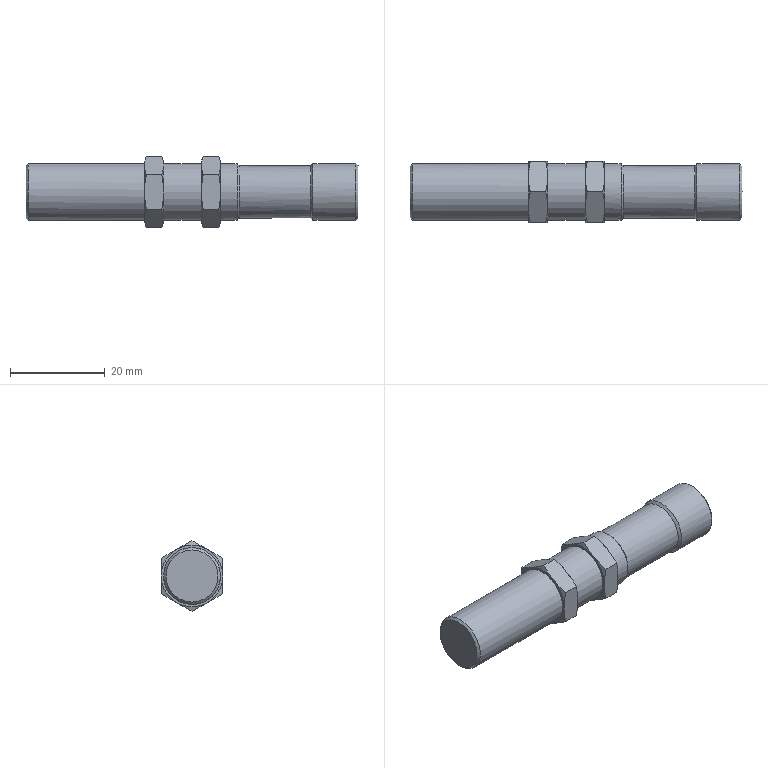Part | NX | features 1605242050 2 | 1 solid | 51 faces | box 70 x 13 x 15.011 mm | volume 7888 mm3 | cone 26 | plane 18 | cylinder 5 | spline 2 | commonest cylinder face diameters 12 x4 11 x1